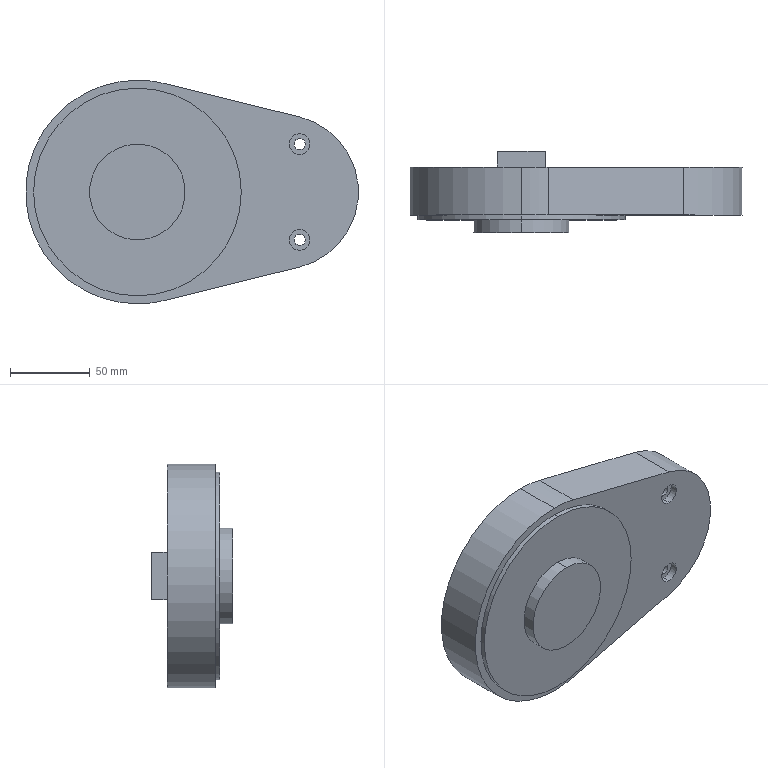Part | SolidWorks | features ICE 3, 3DProfileFeature 1, Extrusion 1, HoleWzd 1 | 1 solid | 29 faces | box 208.413 x 51.01 x 140 mm | volume 738708 mm3 | cylinder 16 | plane 13 | commonest cylinder face diameters 7 x4 13 x4 140 x3 60 x2 130 x2 96.825 x1
STEP:
#1=CARTESIAN_POINT('',(11.612,4.6,-72.5));
#2=VERTEX_POINT('',#1);
#3=CARTESIAN_POINT('',(11.612,4.6,-85.5));
#4=VERTEX_POINT('',#3);
#5=CARTESIAN_POINT('',(11.612,4.6,-79.));
#6=DIRECTION('',(0.,-1.,0.));
#7=DIRECTION('',(0.,0.,-1.));
#8=AXIS2_PLACEMENT_3D('',#5,#6,#7);
#9=CIRCLE('',#8,6.5);
#10=EDGE_CURVE('',#2,#4,#9,.T.);
#11=ORIENTED_EDGE('',*,*,#10,.F.);
#12=CARTESIAN_POINT('',(11.612,0.,-72.5));
#13=VERTEX_POINT('',#12);
#14=CARTESIAN_POINT('',(11.612,0.,-72.5));
#15=DIRECTION('',(0.,-1.,0.));
#16=VECTOR('',#15,1000.);
#17=LINE('',#14,#16);
#18=EDGE_CURVE('',#2,#13,#17,.T.);
#19=ORIENTED_EDGE('',*,*,#18,.T.);
#20=CARTESIAN_POINT('',(11.612,0.,-85.5));
#21=VERTEX_POINT('',#20);
#22=CARTESIAN_POINT('',(11.612,0.,-79.));
#23=DIRECTION('',(0.,-1.,0.));
#24=DIRECTION('',(0.,0.,-1.));
#25=AXIS2_PLACEMENT_3D('',#22,#23,#24);
#26=CIRCLE('',#25,6.5);
#27=EDGE_CURVE('',#13,#21,#26,.T.);
#28=ORIENTED_EDGE('',*,*,#27,.T.);
#29=CARTESIAN_POINT('',(11.612,0.,-85.5));
#30=DIRECTION('',(0.,-1.,0.));
#31=VECTOR('',#30,1000.);
#32=LINE('',#29,#31);
#33=EDGE_CURVE('',#4,#21,#32,.T.);
#34=ORIENTED_EDGE('',*,*,#33,.F.);
#35=EDGE_LOOP('',(#11,#19,#28,#34));
#36=FACE_OUTER_BOUND('',#35,.T.);
#37=CARTESIAN_POINT('',(11.612,0.,-79.));
#38=DIRECTION('',(0.,-1.,0.));
#39=DIRECTION('',(0.,0.,-1.));
#40=AXIS2_PLACEMENT_3D('',#37,#38,#39);
#41=CYLINDRICAL_SURFACE('',#40,6.5);
#42=ADVANCED_FACE('',(#36),#41,.F.);
#43=CARTESIAN_POINT('',(11.612,30.,-82.5));
#44=VERTEX_POINT('',#43);
#45=CARTESIAN_POINT('',(11.612,30.,-75.5));
#46=VERTEX_POINT('',#45);
#47=CARTESIAN_POINT('',(11.612,30.,-79.));
#48=DIRECTION('',(0.,1.,0.));
#49=DIRECTION('',(0.,0.,1.));
#50=AXIS2_PLACEMENT_3D('',#47,#48,#49);
#51=CIRCLE('',#50,3.5);
#52=EDGE_CURVE('',#44,#46,#51,.T.);
#53=ORIENTED_EDGE('',*,*,#52,.T.);
#54=CARTESIAN_POINT('',(11.612,4.6,-75.5));
#55=VERTEX_POINT('',#54);
#56=CARTESIAN_POINT('',(11.612,0.,-75.5));
#57=DIRECTION('',(0.,-1.,0.));
#58=VECTOR('',#57,1000.);
#59=LINE('',#56,#58);
#60=EDGE_CURVE('',#46,#55,#59,.T.);
#61=ORIENTED_EDGE('',*,*,#60,.T.);
#62=CARTESIAN_POINT('',(11.612,4.6,-82.5));
#63=VERTEX_POINT('',#62);
#64=CARTESIAN_POINT('',(11.612,4.6,-79.));
#65=DIRECTION('',(0.,-1.,0.));
#66=DIRECTION('',(0.,0.,-1.));
#67=AXIS2_PLACEMENT_3D('',#64,#65,#66);
#68=CIRCLE('',#67,3.5);
#69=EDGE_CURVE('',#55,#63,#68,.T.);
#70=ORIENTED_EDGE('',*,*,#69,.T.);
#71=CARTESIAN_POINT('',(11.612,0.,-82.5));
#72=DIRECTION('',(0.,-1.,0.));
#73=VECTOR('',#72,1000.);
#74=LINE('',#71,#73);
#75=EDGE_CURVE('',#44,#63,#74,.T.);
#76=ORIENTED_EDGE('',*,*,#75,.F.);
#77=EDGE_LOOP('',(#53,#61,#70,#76));
#78=FACE_OUTER_BOUND('',#77,.T.);
#79=CARTESIAN_POINT('',(11.612,0.,-79.));
#80=DIRECTION('',(0.,-1.,0.));
#81=DIRECTION('',(0.,0.,-1.));
#82=AXIS2_PLACEMENT_3D('',#79,#80,#81);
#83=CYLINDRICAL_SURFACE('',#82,3.5);
#84=ADVANCED_FACE('',(#78),#83,.F.);
#85=CARTESIAN_POINT('',(11.612,4.6,-132.5));
#86=VERTEX_POINT('',#85);
#87=CARTESIAN_POINT('',(11.612,4.6,-145.5));
#88=VERTEX_POINT('',#87);
#89=CARTESIAN_POINT('',(11.612,4.6,-139.));
#90=DIRECTION('',(0.,-1.,0.));
#91=DIRECTION('',(0.,0.,-1.));
#92=AXIS2_PLACEMENT_3D('',#89,#90,#91);
#93=CIRCLE('',#92,6.5);
#94=EDGE_CURVE('',#86,#88,#93,.T.);
#95=ORIENTED_EDGE('',*,*,#94,.F.);
#96=CARTESIAN_POINT('',(11.612,0.,-132.5));
#97=VERTEX_POINT('',#96);
#98=CARTESIAN_POINT('',(11.612,0.,-132.5));
#99=DIRECTION('',(0.,-1.,0.));
#100=VECTOR('',#99,1000.);
#101=LINE('',#98,#100);
#102=EDGE_CURVE('',#86,#97,#101,.T.);
#103=ORIENTED_EDGE('',*,*,#102,.T.);
#104=CARTESIAN_POINT('',(11.612,0.,-145.5));
#105=VERTEX_POINT('',#104);
#106=CARTESIAN_POINT('',(11.612,0.,-139.));
#107=DIRECTION('',(0.,-1.,0.));
#108=DIRECTION('',(0.,0.,-1.));
#109=AXIS2_PLACEMENT_3D('',#106,#107,#108);
#110=CIRCLE('',#109,6.5);
#111=EDGE_CURVE('',#97,#105,#110,.T.);
#112=ORIENTED_EDGE('',*,*,#111,.T.);
#113=CARTESIAN_POINT('',(11.612,0.,-145.5));
#114=DIRECTION('',(0.,-1.,0.));
#115=VECTOR('',#114,1000.);
#116=LINE('',#113,#115);
#117=EDGE_CURVE('',#88,#105,#116,.T.);
#118=ORIENTED_EDGE('',*,*,#117,.F.);
#119=EDGE_LOOP('',(#95,#103,#112,#118));
#120=FACE_OUTER_BOUND('',#119,.T.);
#121=CARTESIAN_POINT('',(11.612,0.,-139.));
#122=DIRECTION('',(0.,-1.,0.));
#123=DIRECTION('',(0.,0.,-1.));
#124=AXIS2_PLACEMENT_3D('',#121,#122,#123);
#125=CYLINDRICAL_SURFACE('',#124,6.5);
#126=ADVANCED_FACE('',(#120),#125,.F.);
#127=CARTESIAN_POINT('',(11.612,30.,-142.5));
#128=VERTEX_POINT('',#127);
#129=CARTESIAN_POINT('',(11.612,30.,-135.5));
#130=VERTEX_POINT('',#129);
#131=CARTESIAN_POINT('',(11.612,30.,-139.));
#132=DIRECTION('',(0.,1.,0.));
#133=DIRECTION('',(0.,0.,1.));
#134=AXIS2_PLACEMENT_3D('',#131,#132,#133);
#135=CIRCLE('',#134,3.5);
#136=EDGE_CURVE('',#128,#130,#135,.T.);
#137=ORIENTED_EDGE('',*,*,#136,.T.);
#138=CARTESIAN_POINT('',(11.612,4.6,-135.5));
#139=VERTEX_POINT('',#138);
#140=CARTESIAN_POINT('',(11.612,0.,-135.5));
#141=DIRECTION('',(0.,-1.,0.));
#142=VECTOR('',#141,1000.);
#143=LINE('',#140,#142);
#144=EDGE_CURVE('',#130,#139,#143,.T.);
#145=ORIENTED_EDGE('',*,*,#144,.T.);
#146=CARTESIAN_POINT('',(11.612,4.6,-142.5));
#147=VERTEX_POINT('',#146);
#148=CARTESIAN_POINT('',(11.612,4.6,-139.));
#149=DIRECTION('',(0.,-1.,0.));
#150=DIRECTION('',(0.,0.,-1.));
#151=AXIS2_PLACEMENT_3D('',#148,#149,#150);
#152=CIRCLE('',#151,3.5);
#153=EDGE_CURVE('',#139,#147,#152,.T.);
#154=ORIENTED_EDGE('',*,*,#153,.T.);
#155=CARTESIAN_POINT('',(11.612,0.,-142.5));
#156=DIRECTION('',(0.,-1.,0.));
#157=VECTOR('',#156,1000.);
#158=LINE('',#155,#157);
#159=EDGE_CURVE('',#128,#147,#158,.T.);
#160=ORIENTED_EDGE('',*,*,#159,.F.);
#161=EDGE_LOOP('',(#137,#145,#154,#160));
#162=FACE_OUTER_BOUND('',#161,.T.);
#163=CARTESIAN_POINT('',(11.612,0.,-139.));
#164=DIRECTION('',(0.,-1.,0.));
#165=DIRECTION('',(0.,0.,-1.));
#166=AXIS2_PLACEMENT_3D('',#163,#164,#165);
#167=CYLINDRICAL_SURFACE('',#166,3.5);
#168=ADVANCED_FACE('',(#162),#167,.F.);
#169=CARTESIAN_POINT('',(-90.,-11.01,-139.));
#170=VERTEX_POINT('',#169);
#171=CARTESIAN_POINT('',(-90.,-11.01,-79.));
#172=VERTEX_POINT('',#171);
#173=CARTESIAN_POINT('',(-90.,-11.01,-109.));
#174=DIRECTION('',(0.,-1.,0.));
#175=DIRECTION('',(0.,0.,-1.));
#176=AXIS2_PLACEMENT_3D('',#173,#174,#175);
#177=CIRCLE('',#176,30.);
#178=EDGE_CURVE('',#170,#172,#177,.T.);
#179=ORIENTED_EDGE('',*,*,#178,.F.);
#180=CARTESIAN_POINT('',(-90.,-3.01,-139.));
#181=VERTEX_POINT('',#180);
#182=CARTESIAN_POINT('',(-90.,-11.01,-139.));
#183=DIRECTION('',(0.,1.,0.));
#184=VECTOR('',#183,1000.);
#185=LINE('',#182,#184);
#186=EDGE_CURVE('',#170,#181,#185,.T.);
#187=ORIENTED_EDGE('',*,*,#186,.T.);
#188=CARTESIAN_POINT('',(-90.,-3.01,-79.));
#189=VERTEX_POINT('',#188);
#190=CARTESIAN_POINT('',(-90.,-3.01,-109.));
#191=DIRECTION('',(0.,-1.,0.));
#192=DIRECTION('',(0.,0.,-1.));
#193=AXIS2_PLACEMENT_3D('',#190,#191,#192);
#194=CIRCLE('',#193,30.);
#195=EDGE_CURVE('',#181,#189,#194,.T.);
#196=ORIENTED_EDGE('',*,*,#195,.T.);
#197=CARTESIAN_POINT('',(-90.,-11.01,-79.));
#198=DIRECTION('',(0.,1.,0.));
#199=VECTOR('',#198,1000.);
#200=LINE('',#197,#199);
#201=EDGE_CURVE('',#172,#189,#200,.T.);
#202=ORIENTED_EDGE('',*,*,#201,.F.);
#203=EDGE_LOOP('',(#179,#187,#196,#202));
#204=FACE_OUTER_BOUND('',#203,.T.);
#205=CARTESIAN_POINT('',(-90.,-11.01,-109.));
#206=DIRECTION('',(0.,1.,0.));
#207=DIRECTION('',(0.,0.,1.));
#208=AXIS2_PLACEMENT_3D('',#205,#206,#207);
#209=CYLINDRICAL_SURFACE('',#208,30.);
#210=ADVANCED_FACE('',(#204),#209,.T.);
#211=CARTESIAN_POINT('',(-90.,-3.01,-174.));
#212=VERTEX_POINT('',#211);
#213=CARTESIAN_POINT('',(-90.,-3.01,-44.));
#214=VERTEX_POINT('',#213);
#215=CARTESIAN_POINT('',(-90.,-3.01,-109.));
#216=DIRECTION('',(0.,-1.,0.));
#217=DIRECTION('',(0.,0.,-1.));
#218=AXIS2_PLACEMENT_3D('',#215,#216,#217);
#219=CIRCLE('',#218,65.);
#220=EDGE_CURVE('',#212,#214,#219,.T.);
#221=ORIENTED_EDGE('',*,*,#220,.F.);
#222=CARTESIAN_POINT('',(-90.,0.,-174.));
#223=VERTEX_POINT('',#222);
#224=CARTESIAN_POINT('',(-90.,-3.01,-174.));
#225=DIRECTION('',(0.,1.,0.));
#226=VECTOR('',#225,1000.);
#227=LINE('',#224,#226);
#228=EDGE_CURVE('',#212,#223,#227,.T.);
#229=ORIENTED_EDGE('',*,*,#228,.T.);
#230=CARTESIAN_POINT('',(-90.,0.,-44.));
#231=VERTEX_POINT('',#230);
#232=CARTESIAN_POINT('',(-90.,0.,-109.));
#233=DIRECTION('',(0.,-1.,0.));
#234=DIRECTION('',(0.,0.,1.));
#235=AXIS2_PLACEMENT_3D('',#232,#233,#234);
#236=CIRCLE('',#235,65.);
#237=EDGE_CURVE('',#223,#231,#236,.T.);
#238=ORIENTED_EDGE('',*,*,#237,.T.);
#239=CARTESIAN_POINT('',(-90.,-3.01,-44.));
#240=DIRECTION('',(0.,1.,0.));
#241=VECTOR('',#240,1000.);
#242=LINE('',#239,#241);
#243=EDGE_CURVE('',#214,#231,#242,.T.);
#244=ORIENTED_EDGE('',*,*,#243,.F.);
#245=EDGE_LOOP('',(#221,#229,#238,#244));
#246=FACE_OUTER_BOUND('',#245,.T.);
#247=CARTESIAN_POINT('',(-90.,-3.01,-109.));
#248=DIRECTION('',(0.,1.,0.));
#249=DIRECTION('',(0.,0.,1.));
#250=AXIS2_PLACEMENT_3D('',#247,#248,#249);
#251=CYLINDRICAL_SURFACE('',#250,65.);
#252=ADVANCED_FACE('',(#246),#251,.T.);
#253=CARTESIAN_POINT('',(-90.,30.,-39.));
#254=VERTEX_POINT('',#253);
#255=CARTESIAN_POINT('',(-73.21,30.,-41.043));
#256=VERTEX_POINT('',#255);
#257=CARTESIAN_POINT('',(-90.,30.,-109.));
#258=DIRECTION('',(0.,1.,0.));
#259=DIRECTION('',(0.,0.,1.));
#260=AXIS2_PLACEMENT_3D('',#257,#258,#259);
#261=CIRCLE('',#260,70.);
#262=EDGE_CURVE('',#254,#256,#261,.T.);
#263=ORIENTED_EDGE('',*,*,#262,.F.);
#264=CARTESIAN_POINT('',(-90.,0.,-39.));
#265=VERTEX_POINT('',#264);
#266=CARTESIAN_POINT('',(-90.,30.,-39.));
#267=DIRECTION('',(0.,-1.,0.));
#268=VECTOR('',#267,1000.);
#269=LINE('',#266,#268);
#270=EDGE_CURVE('',#254,#265,#269,.T.);
#271=ORIENTED_EDGE('',*,*,#270,.T.);
#272=CARTESIAN_POINT('',(-73.21,0.,-41.043));
#273=VERTEX_POINT('',#272);
#274=CARTESIAN_POINT('',(-90.,0.,-109.));
#275=DIRECTION('',(0.,1.,0.));
#276=DIRECTION('',(0.,0.,1.));
#277=AXIS2_PLACEMENT_3D('',#274,#275,#276);
#278=CIRCLE('',#277,70.);
#279=EDGE_CURVE('',#265,#273,#278,.T.);
#280=ORIENTED_EDGE('',*,*,#279,.T.);
#281=CARTESIAN_POINT('',(-73.21,30.,-41.043));
#282=DIRECTION('',(0.,-1.,0.));
#283=VECTOR('',#282,1000.);
#284=LINE('',#281,#283);
#285=EDGE_CURVE('',#256,#273,#284,.T.);
#286=ORIENTED_EDGE('',*,*,#285,.F.);
#287=EDGE_LOOP('',(#263,#271,#280,#286));
#288=FACE_OUTER_BOUND('',#287,.T.);
#289=CARTESIAN_POINT('',(-90.,30.,-109.));
#290=DIRECTION('',(0.,-1.,0.));
#291=DIRECTION('',(0.,0.,-1.));
#292=AXIS2_PLACEMENT_3D('',#289,#290,#291);
#293=CYLINDRICAL_SURFACE('',#292,70.);
#294=ADVANCED_FACE('',(#288),#293,.T.);
#295=ORIENTED_EDGE('',*,*,#270,.F.);
#296=CARTESIAN_POINT('',(-90.,30.,-179.));
#297=VERTEX_POINT('',#296);
#298=CARTESIAN_POINT('',(-90.,30.,-109.));
#299=DIRECTION('',(0.,1.,0.));
#300=DIRECTION('',(0.,0.,1.));
#301=AXIS2_PLACEMENT_3D('',#298,#299,#300);
#302=CIRCLE('',#301,70.);
#303=EDGE_CURVE('',#297,#254,#302,.T.);
#304=ORIENTED_EDGE('',*,*,#303,.F.);
#305=CARTESIAN_POINT('',(-90.,0.,-179.));
#306=VERTEX_POINT('',#305);
#307=CARTESIAN_POINT('',(-90.,30.,-179.));
#308=DIRECTION('',(0.,-1.,0.));
#309=VECTOR('',#308,1000.);
#310=LINE('',#307,#309);
#311=EDGE_CURVE('',#297,#306,#310,.T.);
#312=ORIENTED_EDGE('',*,*,#311,.T.);
#313=CARTESIAN_POINT('',(-90.,0.,-109.));
#314=DIRECTION('',(0.,1.,0.));
#315=DIRECTION('',(0.,0.,1.));
#316=AXIS2_PLACEMENT_3D('',#313,#314,#315);
#317=CIRCLE('',#316,70.);
#318=EDGE_CURVE('',#306,#265,#317,.T.);
#319=ORIENTED_EDGE('',*,*,#318,.T.);
#320=EDGE_LOOP('',(#295,#304,#312,#319));
#321=FACE_OUTER_BOUND('',#320,.T.);
#322=CARTESIAN_POINT('',(-90.,30.,-109.));
#323=DIRECTION('',(0.,-1.,0.));
#324=DIRECTION('',(0.,0.,-1.));
#325=AXIS2_PLACEMENT_3D('',#322,#323,#324);
#326=CYLINDRICAL_SURFACE('',#325,70.);
#327=ADVANCED_FACE('',(#321),#326,.T.);
#328=ORIENTED_EDGE('',*,*,#52,.F.);
#329=CARTESIAN_POINT('',(11.612,30.,-79.));
#330=DIRECTION('',(0.,1.,0.));
#331=DIRECTION('',(0.,0.,1.));
#332=AXIS2_PLACEMENT_3D('',#329,#330,#331);
#333=CIRCLE('',#332,3.5);
#334=EDGE_CURVE('',#46,#44,#333,.T.);
#335=ORIENTED_EDGE('',*,*,#334,.F.);
#336=EDGE_LOOP('',(#328,#335));
#337=FACE_BOUND('',#336,.T.);
#338=ORIENTED_EDGE('',*,*,#136,.F.);
#339=CARTESIAN_POINT('',(11.612,30.,-139.));
#340=DIRECTION('',(0.,1.,0.));
#341=DIRECTION('',(0.,0.,1.));
#342=AXIS2_PLACEMENT_3D('',#339,#340,#341);
#343=CIRCLE('',#342,3.5);
#344=EDGE_CURVE('',#130,#128,#343,.T.);
#345=ORIENTED_EDGE('',*,*,#344,.F.);
#346=EDGE_LOOP('',(#338,#345));
#347=FACE_BOUND('',#346,.T.);
#348=CARTESIAN_POINT('',(11.612,30.,-62.001));
#349=VERTEX_POINT('',#348);
#350=CARTESIAN_POINT('',(-13.769,30.,-55.73));
#351=DIRECTION('',(0.9708,0.,-0.2399));
#352=VECTOR('',#351,1000.);
#353=LINE('',#350,#352);
#354=EDGE_CURVE('',#256,#349,#353,.T.);
#355=ORIENTED_EDGE('',*,*,#354,.T.);
#356=CARTESIAN_POINT('',(11.612,30.,-155.999));
#357=VERTEX_POINT('',#356);
#358=CARTESIAN_POINT('',(0.,30.,-109.));
#359=DIRECTION('',(0.,1.,0.));
#360=DIRECTION('',(0.,0.,1.));
#361=AXIS2_PLACEMENT_3D('',#358,#359,#360);
#362=CIRCLE('',#361,48.413);
#363=EDGE_CURVE('',#349,#357,#362,.T.);
#364=ORIENTED_EDGE('',*,*,#363,.T.);
#365=CARTESIAN_POINT('',(-73.21,30.,-176.957));
#366=VERTEX_POINT('',#365);
#367=CARTESIAN_POINT('',(36.994,30.,-149.728));
#368=DIRECTION('',(0.9708,0.,0.2399));
#369=VECTOR('',#368,1000.);
#370=LINE('',#367,#369);
#371=EDGE_CURVE('',#366,#357,#370,.T.);
#372=ORIENTED_EDGE('',*,*,#371,.F.);
#373=CARTESIAN_POINT('',(-90.,30.,-109.));
#374=DIRECTION('',(0.,1.,0.));
#375=DIRECTION('',(0.,0.,1.));
#376=AXIS2_PLACEMENT_3D('',#373,#374,#375);
#377=CIRCLE('',#376,70.);
#378=EDGE_CURVE('',#366,#297,#377,.T.);
#379=ORIENTED_EDGE('',*,*,#378,.T.);
#380=ORIENTED_EDGE('',*,*,#303,.T.);
#381=ORIENTED_EDGE('',*,*,#262,.T.);
#382=EDGE_LOOP('',(#355,#364,#372,#379,#380,#381));
#383=FACE_OUTER_BOUND('',#382,.T.);
#384=CARTESIAN_POINT('',(-75.,30.,-124.));
#385=VERTEX_POINT('',#384);
#386=CARTESIAN_POINT('',(-105.,30.,-124.));
#387=VERTEX_POINT('',#386);
#388=CARTESIAN_POINT('',(-105.,30.,-124.));
#389=DIRECTION('',(-1.,0.,0.));
#390=VECTOR('',#389,1000.);
#391=LINE('',#388,#390);
#392=EDGE_CURVE('',#385,#387,#391,.T.);
#393=ORIENTED_EDGE('',*,*,#392,.F.);
#394=CARTESIAN_POINT('',(-75.,30.,-94.));
#395=VERTEX_POINT('',#394);
#396=CARTESIAN_POINT('',(-75.,30.,-124.));
#397=DIRECTION('',(0.,0.,-1.));
#398=VECTOR('',#397,1000.);
#399=LINE('',#396,#398);
#400=EDGE_CURVE('',#395,#385,#399,.T.);
#401=ORIENTED_EDGE('',*,*,#400,.F.);
#402=CARTESIAN_POINT('',(-105.,30.,-94.));
#403=VERTEX_POINT('',#402);
#404=CARTESIAN_POINT('',(-105.,30.,-94.));
#405=DIRECTION('',(1.,0.,0.));
#406=VECTOR('',#405,1000.);
#407=LINE('',#404,#406);
#408=EDGE_CURVE('',#403,#395,#407,.T.);
#409=ORIENTED_EDGE('',*,*,#408,.F.);
#410=CARTESIAN_POINT('',(-105.,30.,-124.));
#411=DIRECTION('',(0.,0.,1.));
#412=VECTOR('',#411,1000.);
#413=LINE('',#410,#412);
#414=EDGE_CURVE('',#387,#403,#413,.T.);
#415=ORIENTED_EDGE('',*,*,#414,.F.);
#416=EDGE_LOOP('',(#393,#401,#409,#415));
#417=FACE_BOUND('',#416,.T.);
#418=CARTESIAN_POINT('',(0.,30.,0.));
#419=DIRECTION('',(0.,1.,0.));
#420=DIRECTION('',(0.,0.,1.));
#421=AXIS2_PLACEMENT_3D('',#418,#419,#420);
#422=PLANE('',#421);
#423=ADVANCED_FACE('',(#337,#347,#383,#417),#422,.T.);
#424=CARTESIAN_POINT('',(11.612,0.,-62.001));
#425=VERTEX_POINT('',#424);
#426=CARTESIAN_POINT('',(-13.769,0.,-55.73));
#427=DIRECTION('',(0.9708,0.,-0.2399));
#428=VECTOR('',#427,1000.);
#429=LINE('',#426,#428);
#430=EDGE_CURVE('',#273,#425,#429,.T.);
#431=ORIENTED_EDGE('',*,*,#430,.T.);
#432=CARTESIAN_POINT('',(11.612,30.,-62.001));
#433=DIRECTION('',(0.,-1.,0.));
#434=VECTOR('',#433,1000.);
#435=LINE('',#432,#434);
#436=EDGE_CURVE('',#349,#425,#435,.T.);
#437=ORIENTED_EDGE('',*,*,#436,.F.);
#438=ORIENTED_EDGE('',*,*,#354,.F.);
#439=ORIENTED_EDGE('',*,*,#285,.T.);
#440=EDGE_LOOP('',(#431,#437,#438,#439));
#441=FACE_OUTER_BOUND('',#440,.T.);
#442=CARTESIAN_POINT('',(-13.769,30.,-55.73));
#443=DIRECTION('',(-0.2399,0.,-0.9708));
#444=DIRECTION('',(-0.9708,0.,0.2399));
#445=AXIS2_PLACEMENT_3D('',#442,#443,#444);
#446=PLANE('',#445);
#447=ADVANCED_FACE('',(#441),#446,.F.);
#448=CARTESIAN_POINT('',(11.612,0.,-155.999));
#449=VERTEX_POINT('',#448);
#450=CARTESIAN_POINT('',(0.,0.,-109.));
#451=DIRECTION('',(0.,1.,0.));
#452=DIRECTION('',(0.,0.,1.));
#453=AXIS2_PLACEMENT_3D('',#450,#451,#452);
#454=CIRCLE('',#453,48.413);
#455=EDGE_CURVE('',#425,#449,#454,.T.);
#456=ORIENTED_EDGE('',*,*,#455,.T.);
#457=CARTESIAN_POINT('',(11.612,30.,-155.999));
#458=DIRECTION('',(0.,-1.,0.));
#459=VECTOR('',#458,1000.);
#460=LINE('',#457,#459);
#461=EDGE_CURVE('',#357,#449,#460,.T.);
#462=ORIENTED_EDGE('',*,*,#461,.F.);
#463=ORIENTED_EDGE('',*,*,#363,.F.);
#464=ORIENTED_EDGE('',*,*,#436,.T.);
#465=EDGE_LOOP('',(#456,#462,#463,#464));
#466=FACE_OUTER_BOUND('',#465,.T.);
#467=CARTESIAN_POINT('',(0.,30.,-109.));
#468=DIRECTION('',(0.,-1.,0.));
#469=DIRECTION('',(0.,0.,-1.));
#470=AXIS2_PLACEMENT_3D('',#467,#468,#469);
#471=CYLINDRICAL_SURFACE('',#470,48.413);
#472=ADVANCED_FACE('',(#466),#471,.T.);
#473=CARTESIAN_POINT('',(-73.21,0.,-176.957));
#474=VERTEX_POINT('',#473);
#475=CARTESIAN_POINT('',(36.994,0.,-149.728));
#476=DIRECTION('',(0.9708,0.,0.2399));
#477=VECTOR('',#476,1000.);
#478=LINE('',#475,#477);
#479=EDGE_CURVE('',#474,#449,#478,.T.);
#480=ORIENTED_EDGE('',*,*,#479,.F.);
#481=CARTESIAN_POINT('',(-73.21,30.,-176.957));
#482=DIRECTION('',(0.,-1.,0.));
#483=VECTOR('',#482,1000.);
#484=LINE('',#481,#483);
#485=EDGE_CURVE('',#366,#474,#484,.T.);
#486=ORIENTED_EDGE('',*,*,#485,.F.);
#487=ORIENTED_EDGE('',*,*,#371,.T.);
#488=ORIENTED_EDGE('',*,*,#461,.T.);
#489=EDGE_LOOP('',(#480,#486,#487,#488));
#490=FACE_OUTER_BOUND('',#489,.T.);
#491=CARTESIAN_POINT('',(36.994,30.,-149.728));
#492=DIRECTION('',(0.2399,0.,-0.9708));
#493=DIRECTION('',(-0.9708,0.,-0.2399));
#494=AXIS2_PLACEMENT_3D('',#491,#492,#493);
#495=PLANE('',#494);
#496=ADVANCED_FACE('',(#490),#495,.T.);
#497=ORIENTED_EDGE('',*,*,#311,.F.);
#498=ORIENTED_EDGE('',*,*,#378,.F.);
#499=ORIENTED_EDGE('',*,*,#485,.T.);
#500=CARTESIAN_POINT('',(-90.,0.,-109.));
#501=DIRECTION('',(0.,1.,0.));
#502=DIRECTION('',(0.,0.,1.));
#503=AXIS2_PLACEMENT_3D('',#500,#501,#502);
#504=CIRCLE('',#503,70.);
#505=EDGE_CURVE('',#474,#306,#504,.T.);
#506=ORIENTED_EDGE('',*,*,#505,.T.);
#507=EDGE_LOOP('',(#497,#498,#499,#506));
#508=FACE_OUTER_BOUND('',#507,.T.);
#509=CARTESIAN_POINT('',(-90.,30.,-109.));
#510=DIRECTION('',(0.,-1.,0.));
#511=DIRECTION('',(0.,0.,-1.));
#512=AXIS2_PLACEMENT_3D('',#509,#510,#511);
#513=CYLINDRICAL_SURFACE('',#512,70.);
#514=ADVANCED_FACE('',(#508),#513,.T.);
#515=CARTESIAN_POINT('',(11.612,0.,-79.));
#516=DIRECTION('',(0.,-1.,0.));
#517=DIRECTION('',(0.,0.,-1.));
#518=AXIS2_PLACEMENT_3D('',#515,#516,#517);
#519=CIRCLE('',#518,6.5);
#520=EDGE_CURVE('',#21,#13,#519,.T.);
#521=ORIENTED_EDGE('',*,*,#520,.F.);
#522=ORIENTED_EDGE('',*,*,#27,.F.);
#523=EDGE_LOOP('',(#521,#522));
#524=FACE_BOUND('',#523,.T.);
#525=CARTESIAN_POINT('',(11.612,0.,-139.));
#526=DIRECTION('',(0.,-1.,0.));
#527=DIRECTION('',(0.,0.,-1.));
#528=AXIS2_PLACEMENT_3D('',#525,#526,#527);
#529=CIRCLE('',#528,6.5);
#530=EDGE_CURVE('',#105,#97,#529,.T.);
#531=ORIENTED_EDGE('',*,*,#530,.F.);
#532=ORIENTED_EDGE('',*,*,#111,.F.);
#533=EDGE_LOOP('',(#531,#532));
#534=FACE_BOUND('',#533,.T.);
#535=CARTESIAN_POINT('',(-90.,0.,-109.));
#536=DIRECTION('',(0.,-1.,0.));
#537=DIRECTION('',(0.,0.,1.));
#538=AXIS2_PLACEMENT_3D('',#535,#536,#537);
#539=CIRCLE('',#538,65.);
#540=EDGE_CURVE('',#231,#223,#539,.T.);
#541=ORIENTED_EDGE('',*,*,#540,.F.);
#542=ORIENTED_EDGE('',*,*,#237,.F.);
#543=EDGE_LOOP('',(#541,#542));
#544=FACE_BOUND('',#543,.T.);
#545=ORIENTED_EDGE('',*,*,#430,.F.);
#546=ORIENTED_EDGE('',*,*,#279,.F.);
#547=ORIENTED_EDGE('',*,*,#318,.F.);
#548=ORIENTED_EDGE('',*,*,#505,.F.);
#549=ORIENTED_EDGE('',*,*,#479,.T.);
#550=ORIENTED_EDGE('',*,*,#455,.F.);
#551=EDGE_LOOP('',(#545,#546,#547,#548,#549,#550));
#552=FACE_OUTER_BOUND('',#551,.T.);
#553=CARTESIAN_POINT('',(0.,0.,0.));
#554=DIRECTION('',(0.,1.,0.));
#555=DIRECTION('',(0.,0.,1.));
#556=AXIS2_PLACEMENT_3D('',#553,#554,#555);
#557=PLANE('',#556);
#558=ADVANCED_FACE('',(#524,#534,#544,#552),#557,.F.);
#559=ORIENTED_EDGE('',*,*,#400,.T.);
#560=CARTESIAN_POINT('',(-75.,40.,-124.));
#561=VERTEX_POINT('',#560);
#562=CARTESIAN_POINT('',(-75.,40.,-124.));
#563=DIRECTION('',(0.,-1.,0.));
#564=VECTOR('',#563,1000.);
#565=LINE('',#562,#564);
#566=EDGE_CURVE('',#561,#385,#565,.T.);
#567=ORIENTED_EDGE('',*,*,#566,.F.);
#568=CARTESIAN_POINT('',(-75.,40.,-94.));
#569=VERTEX_POINT('',#568);
#570=CARTESIAN_POINT('',(-75.,40.,-124.));
#571=DIRECTION('',(0.,0.,-1.));
#572=VECTOR('',#571,1000.);
#573=LINE('',#570,#572);
#574=EDGE_CURVE('',#569,#561,#573,.T.);
#575=ORIENTED_EDGE('',*,*,#574,.F.);
#576=CARTESIAN_POINT('',(-75.,40.,-94.));
#577=DIRECTION('',(0.,-1.,0.));
#578=VECTOR('',#577,1000.);
#579=LINE('',#576,#578);
#580=EDGE_CURVE('',#569,#395,#579,.T.);
#581=ORIENTED_EDGE('',*,*,#580,.T.);
#582=EDGE_LOOP('',(#559,#567,#575,#581));
#583=FACE_OUTER_BOUND('',#582,.T.);
#584=CARTESIAN_POINT('',(-75.,40.,-124.));
#585=DIRECTION('',(-1.,0.,0.));
#586=DIRECTION('',(0.,0.,1.));
#587=AXIS2_PLACEMENT_3D('',#584,#585,#586);
#588=PLANE('',#587);
#589=ADVANCED_FACE('',(#583),#588,.F.);
#590=ORIENTED_EDGE('',*,*,#392,.T.);
#591=CARTESIAN_POINT('',(-105.,40.,-124.));
#592=VERTEX_POINT('',#591);
#593=CARTESIAN_POINT('',(-105.,40.,-124.));
#594=DIRECTION('',(0.,-1.,0.));
#595=VECTOR('',#594,1000.);
#596=LINE('',#593,#595);
#597=EDGE_CURVE('',#592,#387,#596,.T.);
#598=ORIENTED_EDGE('',*,*,#597,.F.);
#599=CARTESIAN_POINT('',(-105.,40.,-124.));
#600=DIRECTION('',(-1.,0.,0.));
#601=VECTOR('',#600,1000.);
#602=LINE('',#599,#601);
#603=EDGE_CURVE('',#561,#592,#602,.T.);
#604=ORIENTED_EDGE('',*,*,#603,.F.);
#605=ORIENTED_EDGE('',*,*,#566,.T.);
#606=EDGE_LOOP('',(#590,#598,#604,#605));
#607=FACE_OUTER_BOUND('',#606,.T.);
#608=CARTESIAN_POINT('',(-105.,40.,-124.));
#609=DIRECTION('',(0.,0.,1.));
#610=DIRECTION('',(1.,0.,0.));
#611=AXIS2_PLACEMENT_3D('',#608,#609,#610);
#612=PLANE('',#611);
#613=ADVANCED_FACE('',(#607),#612,.F.);
#614=ORIENTED_EDGE('',*,*,#414,.T.);
#615=CARTESIAN_POINT('',(-105.,40.,-94.));
#616=VERTEX_POINT('',#615);
#617=CARTESIAN_POINT('',(-105.,40.,-94.));
#618=DIRECTION('',(0.,-1.,0.));
#619=VECTOR('',#618,1000.);
#620=LINE('',#617,#619);
#621=EDGE_CURVE('',#616,#403,#620,.T.);
#622=ORIENTED_EDGE('',*,*,#621,.F.);
#623=CARTESIAN_POINT('',(-105.,40.,-124.));
#624=DIRECTION('',(0.,0.,1.));
#625=VECTOR('',#624,1000.);
#626=LINE('',#623,#625);
#627=EDGE_CURVE('',#592,#616,#626,.T.);
#628=ORIENTED_EDGE('',*,*,#627,.F.);
#629=ORIENTED_EDGE('',*,*,#597,.T.);
#630=EDGE_LOOP('',(#614,#622,#628,#629));
#631=FACE_OUTER_BOUND('',#630,.T.);
#632=CARTESIAN_POINT('',(-105.,40.,-124.));
#633=DIRECTION('',(1.,0.,0.));
#634=DIRECTION('',(0.,0.,-1.));
#635=AXIS2_PLACEMENT_3D('',#632,#633,#634);
#636=PLANE('',#635);
#637=ADVANCED_FACE('',(#631),#636,.F.);
#638=ORIENTED_EDGE('',*,*,#408,.T.);
#639=ORIENTED_EDGE('',*,*,#580,.F.);
#640=CARTESIAN_POINT('',(-105.,40.,-94.));
#641=DIRECTION('',(1.,0.,0.));
#642=VECTOR('',#641,1000.);
#643=LINE('',#640,#642);
#644=EDGE_CURVE('',#616,#569,#643,.T.);
#645=ORIENTED_EDGE('',*,*,#644,.F.);
#646=ORIENTED_EDGE('',*,*,#621,.T.);
#647=EDGE_LOOP('',(#638,#639,#645,#646));
#648=FACE_OUTER_BOUND('',#647,.T.);
#649=CARTESIAN_POINT('',(-105.,40.,-94.));
#650=DIRECTION('',(0.,0.,-1.));
#651=DIRECTION('',(-1.,0.,0.));
#652=AXIS2_PLACEMENT_3D('',#649,#650,#651);
#653=PLANE('',#652);
#654=ADVANCED_FACE('',(#648),#653,.F.);
#655=ORIENTED_EDGE('',*,*,#574,.T.);
#656=ORIENTED_EDGE('',*,*,#603,.T.);
#657=ORIENTED_EDGE('',*,*,#627,.T.);
#658=ORIENTED_EDGE('',*,*,#644,.T.);
#659=EDGE_LOOP('',(#655,#656,#657,#658));
#660=FACE_OUTER_BOUND('',#659,.T.);
#661=CARTESIAN_POINT('',(0.,40.,0.));
#662=DIRECTION('',(0.,1.,0.));
#663=DIRECTION('',(0.,0.,1.));
#664=AXIS2_PLACEMENT_3D('',#661,#662,#663);
#665=PLANE('',#664);
#666=ADVANCED_FACE('',(#660),#665,.T.);
#667=ORIENTED_EDGE('',*,*,#228,.F.);
#668=CARTESIAN_POINT('',(-90.,-3.01,-109.));
#669=DIRECTION('',(0.,-1.,0.));
#670=DIRECTION('',(0.,0.,-1.));
#671=AXIS2_PLACEMENT_3D('',#668,#669,#670);
#672=CIRCLE('',#671,65.);
#673=EDGE_CURVE('',#214,#212,#672,.T.);
#674=ORIENTED_EDGE('',*,*,#673,.F.);
#675=ORIENTED_EDGE('',*,*,#243,.T.);
#676=ORIENTED_EDGE('',*,*,#540,.T.);
#677=EDGE_LOOP('',(#667,#674,#675,#676));
#678=FACE_OUTER_BOUND('',#677,.T.);
#679=CARTESIAN_POINT('',(-90.,-3.01,-109.));
#680=DIRECTION('',(0.,1.,0.));
#681=DIRECTION('',(0.,0.,1.));
#682=AXIS2_PLACEMENT_3D('',#679,#680,#681);
#683=CYLINDRICAL_SURFACE('',#682,65.);
#684=ADVANCED_FACE('',(#678),#683,.T.);
#685=CARTESIAN_POINT('',(-90.,-3.01,-109.));
#686=DIRECTION('',(0.,-1.,0.));
#687=DIRECTION('',(0.,0.,-1.));
#688=AXIS2_PLACEMENT_3D('',#685,#686,#687);
#689=CIRCLE('',#688,30.);
#690=EDGE_CURVE('',#189,#181,#689,.T.);
#691=ORIENTED_EDGE('',*,*,#690,.F.);
#692=ORIENTED_EDGE('',*,*,#195,.F.);
#693=EDGE_LOOP('',(#691,#692));
#694=FACE_BOUND('',#693,.T.);
#695=ORIENTED_EDGE('',*,*,#673,.T.);
#696=ORIENTED_EDGE('',*,*,#220,.T.);
#697=EDGE_LOOP('',(#695,#696));
#698=FACE_OUTER_BOUND('',#697,.T.);
#699=CARTESIAN_POINT('',(-90.,-3.01,-109.));
#700=DIRECTION('',(0.,-1.,0.));
#701=DIRECTION('',(0.,0.,-1.));
#702=AXIS2_PLACEMENT_3D('',#699,#700,#701);
#703=PLANE('',#702);
#704=ADVANCED_FACE('',(#694,#698),#703,.T.);
#705=ORIENTED_EDGE('',*,*,#186,.F.);
#706=CARTESIAN_POINT('',(-90.,-11.01,-109.));
#707=DIRECTION('',(0.,-1.,0.));
#708=DIRECTION('',(0.,0.,-1.));
#709=AXIS2_PLACEMENT_3D('',#706,#707,#708);
#710=CIRCLE('',#709,30.);
#711=EDGE_CURVE('',#172,#170,#710,.T.);
#712=ORIENTED_EDGE('',*,*,#711,.F.);
#713=ORIENTED_EDGE('',*,*,#201,.T.);
#714=ORIENTED_EDGE('',*,*,#690,.T.);
#715=EDGE_LOOP('',(#705,#712,#713,#714));
#716=FACE_OUTER_BOUND('',#715,.T.);
#717=CARTESIAN_POINT('',(-90.,-11.01,-109.));
#718=DIRECTION('',(0.,1.,0.));
#719=DIRECTION('',(0.,0.,1.));
#720=AXIS2_PLACEMENT_3D('',#717,#718,#719);
#721=CYLINDRICAL_SURFACE('',#720,30.);
#722=ADVANCED_FACE('',(#716),#721,.T.);
#723=ORIENTED_EDGE('',*,*,#711,.T.);
#724=ORIENTED_EDGE('',*,*,#178,.T.);
#725=EDGE_LOOP('',(#723,#724));
#726=FACE_OUTER_BOUND('',#725,.T.);
#727=CARTESIAN_POINT('',(-90.,-11.01,-109.));
#728=DIRECTION('',(0.,-1.,0.));
#729=DIRECTION('',(0.,0.,-1.));
#730=AXIS2_PLACEMENT_3D('',#727,#728,#729);
#731=PLANE('',#730);
#732=ADVANCED_FACE('',(#726),#731,.T.);
#733=ORIENTED_EDGE('',*,*,#144,.F.);
#734=ORIENTED_EDGE('',*,*,#344,.T.);
#735=ORIENTED_EDGE('',*,*,#159,.T.);
#736=CARTESIAN_POINT('',(11.612,4.6,-139.));
#737=DIRECTION('',(0.,-1.,0.));
#738=DIRECTION('',(0.,0.,-1.));
#739=AXIS2_PLACEMENT_3D('',#736,#737,#738);
#740=CIRCLE('',#739,3.5);
#741=EDGE_CURVE('',#147,#139,#740,.T.);
#742=ORIENTED_EDGE('',*,*,#741,.T.);
#743=EDGE_LOOP('',(#733,#734,#735,#742));
#744=FACE_OUTER_BOUND('',#743,.T.);
#745=CARTESIAN_POINT('',(11.612,0.,-139.));
#746=DIRECTION('',(0.,-1.,0.));
#747=DIRECTION('',(0.,0.,-1.));
#748=AXIS2_PLACEMENT_3D('',#745,#746,#747);
#749=CYLINDRICAL_SURFACE('',#748,3.5);
#750=ADVANCED_FACE('',(#744),#749,.F.);
#751=ORIENTED_EDGE('',*,*,#741,.F.);
#752=ORIENTED_EDGE('',*,*,#153,.F.);
#753=EDGE_LOOP('',(#751,#752));
#754=FACE_BOUND('',#753,.T.);
#755=CARTESIAN_POINT('',(11.612,4.6,-139.));
#756=DIRECTION('',(0.,-1.,0.));
#757=DIRECTION('',(0.,0.,-1.));
#758=AXIS2_PLACEMENT_3D('',#755,#756,#757);
#759=CIRCLE('',#758,6.5);
#760=EDGE_CURVE('',#88,#86,#759,.T.);
#761=ORIENTED_EDGE('',*,*,#760,.T.);
#762=ORIENTED_EDGE('',*,*,#94,.T.);
#763=EDGE_LOOP('',(#761,#762));
#764=FACE_OUTER_BOUND('',#763,.T.);
#765=CARTESIAN_POINT('',(15.112,4.6,-139.));
#766=DIRECTION('',(0.,1.,0.));
#767=DIRECTION('',(0.,0.,1.));
#768=AXIS2_PLACEMENT_3D('',#765,#766,#767);
#769=PLANE('',#768);
#770=ADVANCED_FACE('',(#754,#764),#769,.F.);
#771=ORIENTED_EDGE('',*,*,#102,.F.);
#772=ORIENTED_EDGE('',*,*,#760,.F.);
#773=ORIENTED_EDGE('',*,*,#117,.T.);
#774=ORIENTED_EDGE('',*,*,#530,.T.);
#775=EDGE_LOOP('',(#771,#772,#773,#774));
#776=FACE_OUTER_BOUND('',#775,.T.);
#777=CARTESIAN_POINT('',(11.612,0.,-139.));
#778=DIRECTION('',(0.,-1.,0.));
#779=DIRECTION('',(0.,0.,-1.));
#780=AXIS2_PLACEMENT_3D('',#777,#778,#779);
#781=CYLINDRICAL_SURFACE('',#780,6.5);
#782=ADVANCED_FACE('',(#776),#781,.F.);
#783=ORIENTED_EDGE('',*,*,#60,.F.);
#784=ORIENTED_EDGE('',*,*,#334,.T.);
#785=ORIENTED_EDGE('',*,*,#75,.T.);
#786=CARTESIAN_POINT('',(11.612,4.6,-79.));
#787=DIRECTION('',(0.,-1.,0.));
#788=DIRECTION('',(0.,0.,-1.));
#789=AXIS2_PLACEMENT_3D('',#786,#787,#788);
#790=CIRCLE('',#789,3.5);
#791=EDGE_CURVE('',#63,#55,#790,.T.);
#792=ORIENTED_EDGE('',*,*,#791,.T.);
#793=EDGE_LOOP('',(#783,#784,#785,#792));
#794=FACE_OUTER_BOUND('',#793,.T.);
#795=CARTESIAN_POINT('',(11.612,0.,-79.));
#796=DIRECTION('',(0.,-1.,0.));
#797=DIRECTION('',(0.,0.,-1.));
#798=AXIS2_PLACEMENT_3D('',#795,#796,#797);
#799=CYLINDRICAL_SURFACE('',#798,3.5);
#800=ADVANCED_FACE('',(#794),#799,.F.);
#801=ORIENTED_EDGE('',*,*,#791,.F.);
#802=ORIENTED_EDGE('',*,*,#69,.F.);
#803=EDGE_LOOP('',(#801,#802));
#804=FACE_BOUND('',#803,.T.);
#805=CARTESIAN_POINT('',(11.612,4.6,-79.));
#806=DIRECTION('',(0.,-1.,0.));
#807=DIRECTION('',(0.,0.,-1.));
#808=AXIS2_PLACEMENT_3D('',#805,#806,#807);
#809=CIRCLE('',#808,6.5);
#810=EDGE_CURVE('',#4,#2,#809,.T.);
#811=ORIENTED_EDGE('',*,*,#810,.T.);
#812=ORIENTED_EDGE('',*,*,#10,.T.);
#813=EDGE_LOOP('',(#811,#812));
#814=FACE_OUTER_BOUND('',#813,.T.);
#815=CARTESIAN_POINT('',(15.112,4.6,-79.));
#816=DIRECTION('',(0.,1.,0.));
#817=DIRECTION('',(0.,0.,1.));
#818=AXIS2_PLACEMENT_3D('',#815,#816,#817);
#819=PLANE('',#818);
#820=ADVANCED_FACE('',(#804,#814),#819,.F.);
#821=ORIENTED_EDGE('',*,*,#18,.F.);
#822=ORIENTED_EDGE('',*,*,#810,.F.);
#823=ORIENTED_EDGE('',*,*,#33,.T.);
#824=ORIENTED_EDGE('',*,*,#520,.T.);
#825=EDGE_LOOP('',(#821,#822,#823,#824));
#826=FACE_OUTER_BOUND('',#825,.T.);
#827=CARTESIAN_POINT('',(11.612,0.,-79.));
#828=DIRECTION('',(0.,-1.,0.));
#829=DIRECTION('',(0.,0.,-1.));
#830=AXIS2_PLACEMENT_3D('',#827,#828,#829);
#831=CYLINDRICAL_SURFACE('',#830,6.5);
#832=ADVANCED_FACE('',(#826),#831,.F.);
#833=CLOSED_SHELL('',(#42,#84,#126,#168,#210,#252,#294,#327,#423,#447,#472,#496,#514,#558,#589,#613,#637,#654,#666,#684,#704,#722,#732,#750,#770,#782,#800,#820,#832));
#834=MANIFOLD_SOLID_BREP('',#833);
#835=CARTESIAN_POINT('',(0.,0.,0.));
#836=DIRECTION('',(0.,0.,1.));
#837=DIRECTION('',(1.,0.,0.));
#838=AXIS2_PLACEMENT_3D('',#835,#836,#837);
#839=(LENGTH_UNIT()NAMED_UNIT(*)SI_UNIT(.MILLI.,.METRE.));
#840=UNCERTAINTY_MEASURE_WITH_UNIT(LENGTH_MEASURE(0.00001),#839,'','');
#841=(NAMED_UNIT(*)PLANE_ANGLE_UNIT()SI_UNIT($,.RADIAN.));
#842=(NAMED_UNIT(*)SI_UNIT($,.STERADIAN.)SOLID_ANGLE_UNIT());
#843=(GEOMETRIC_REPRESENTATION_CONTEXT(3)GLOBAL_UNCERTAINTY_ASSIGNED_CONTEXT((#840))GLOBAL_UNIT_ASSIGNED_CONTEXT((#839,#841,#842))REPRESENTATION_CONTEXT('',''));
#844=ADVANCED_BREP_SHAPE_REPRESENTATION('',(#834,#838),#843);